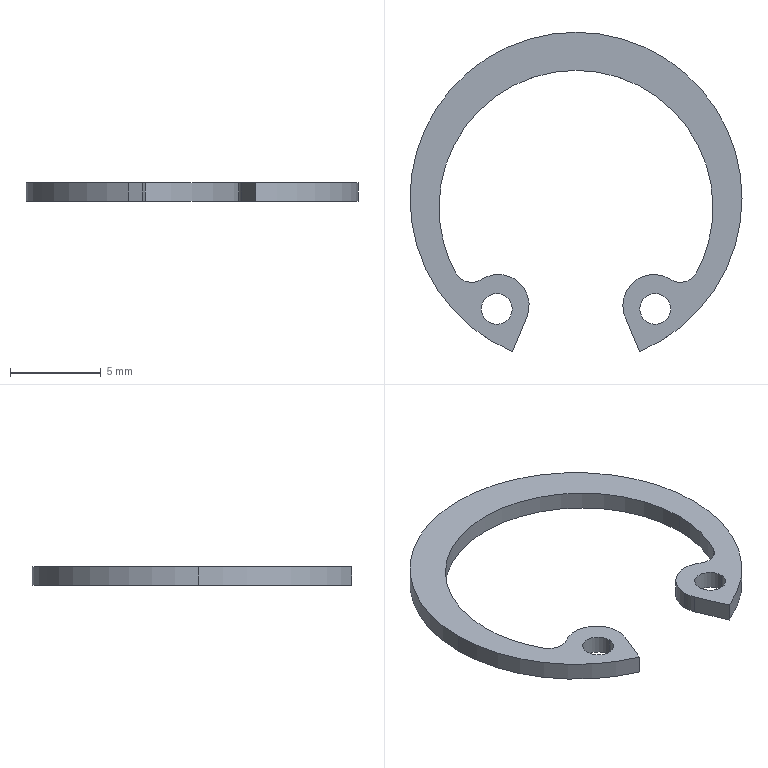Part | NX | features BREP 1 | 1 solid | 19 faces | box 18.3 x 17.603 x 1 mm | volume 85.781 mm3 | cylinder 15 | plane 4 | commonest cylinder face diameters 1.7 x4 3.4 x3 15.1 x3 18.3 x3 2 x2
STEP:
#1=CARTESIAN_POINT('',(-2.713,-6.549,-0.5));
#2=VERTEX_POINT('',#1);
#3=CARTESIAN_POINT('',(-5.208,-4.472,-0.5));
#4=VERTEX_POINT('',#3);
#5=CARTESIAN_POINT('',(-4.283,-5.899,-0.5));
#6=DIRECTION('',(0.,0.,1.));
#7=DIRECTION('',(1.,0.,0.));
#8=AXIS2_PLACEMENT_3D('',#5,#6,#7);
#9=CIRCLE('',#8,1.7);
#10=EDGE_CURVE('',#2,#4,#9,.T.);
#11=ORIENTED_EDGE('',*,*,#10,.F.);
#12=CARTESIAN_POINT('',(-3.502,-8.453,-0.5));
#13=VERTEX_POINT('',#12);
#14=CARTESIAN_POINT('',(-2.713,-6.549,-0.5));
#15=DIRECTION('',(0.3827,0.9239,0.));
#16=VECTOR('',#15,1000.);
#17=LINE('',#14,#16);
#18=EDGE_CURVE('',#13,#2,#17,.T.);
#19=ORIENTED_EDGE('',*,*,#18,.F.);
#20=CARTESIAN_POINT('',(-9.15,0.,-0.5));
#21=VERTEX_POINT('',#20);
#22=CARTESIAN_POINT('',(0.,0.,-0.5));
#23=DIRECTION('',(0.,0.,1.));
#24=DIRECTION('',(1.,0.,0.));
#25=AXIS2_PLACEMENT_3D('',#22,#23,#24);
#26=CIRCLE('',#25,9.15);
#27=EDGE_CURVE('',#21,#13,#26,.T.);
#28=ORIENTED_EDGE('',*,*,#27,.F.);
#29=CARTESIAN_POINT('',(9.15,0.,-0.5));
#30=VERTEX_POINT('',#29);
#31=CARTESIAN_POINT('',(0.,0.,-0.5));
#32=DIRECTION('',(0.,0.,1.));
#33=DIRECTION('',(1.,0.,0.));
#34=AXIS2_PLACEMENT_3D('',#31,#32,#33);
#35=CIRCLE('',#34,9.15);
#36=EDGE_CURVE('',#30,#21,#35,.T.);
#37=ORIENTED_EDGE('',*,*,#36,.F.);
#38=CARTESIAN_POINT('',(3.502,-8.453,-0.5));
#39=VERTEX_POINT('',#38);
#40=CARTESIAN_POINT('',(0.,0.,-0.5));
#41=DIRECTION('',(0.,0.,1.));
#42=DIRECTION('',(1.,0.,0.));
#43=AXIS2_PLACEMENT_3D('',#40,#41,#42);
#44=CIRCLE('',#43,9.15);
#45=EDGE_CURVE('',#39,#30,#44,.T.);
#46=ORIENTED_EDGE('',*,*,#45,.F.);
#47=CARTESIAN_POINT('',(2.713,-6.549,-0.5));
#48=VERTEX_POINT('',#47);
#49=CARTESIAN_POINT('',(2.713,-6.549,-0.5));
#50=DIRECTION('',(0.3827,-0.9239,0.));
#51=VECTOR('',#50,1000.);
#52=LINE('',#49,#51);
#53=EDGE_CURVE('',#48,#39,#52,.T.);
#54=ORIENTED_EDGE('',*,*,#53,.F.);
#55=CARTESIAN_POINT('',(2.583,-5.899,-0.5));
#56=VERTEX_POINT('',#55);
#57=CARTESIAN_POINT('',(4.283,-5.899,-0.5));
#58=DIRECTION('',(0.,0.,1.));
#59=DIRECTION('',(-1.,0.,0.));
#60=AXIS2_PLACEMENT_3D('',#57,#58,#59);
#61=CIRCLE('',#60,1.7);
#62=EDGE_CURVE('',#56,#48,#61,.T.);
#63=ORIENTED_EDGE('',*,*,#62,.F.);
#64=CARTESIAN_POINT('',(5.208,-4.472,-0.5));
#65=VERTEX_POINT('',#64);
#66=CARTESIAN_POINT('',(4.283,-5.899,-0.5));
#67=DIRECTION('',(0.,0.,1.));
#68=DIRECTION('',(-1.,0.,0.));
#69=AXIS2_PLACEMENT_3D('',#66,#67,#68);
#70=CIRCLE('',#69,1.7);
#71=EDGE_CURVE('',#65,#56,#70,.T.);
#72=ORIENTED_EDGE('',*,*,#71,.F.);
#73=CARTESIAN_POINT('',(6.63,-4.112,-0.5));
#74=VERTEX_POINT('',#73);
#75=CARTESIAN_POINT('',(5.752,-3.633,-0.5));
#76=DIRECTION('',(0.,0.,-1.));
#77=DIRECTION('',(1.,0.,0.));
#78=AXIS2_PLACEMENT_3D('',#75,#76,#77);
#79=CIRCLE('',#78,1.);
#80=EDGE_CURVE('',#74,#65,#79,.T.);
#81=ORIENTED_EDGE('',*,*,#80,.F.);
#82=CARTESIAN_POINT('',(7.55,-0.5,-0.5));
#83=VERTEX_POINT('',#82);
#84=CARTESIAN_POINT('',(0.,-0.5,-0.5));
#85=DIRECTION('',(0.,0.,-1.));
#86=DIRECTION('',(1.,0.,0.));
#87=AXIS2_PLACEMENT_3D('',#84,#85,#86);
#88=CIRCLE('',#87,7.55);
#89=EDGE_CURVE('',#83,#74,#88,.T.);
#90=ORIENTED_EDGE('',*,*,#89,.F.);
#91=CARTESIAN_POINT('',(-7.55,-0.5,-0.5));
#92=VERTEX_POINT('',#91);
#93=CARTESIAN_POINT('',(0.,-0.5,-0.5));
#94=DIRECTION('',(0.,0.,-1.));
#95=DIRECTION('',(1.,0.,0.));
#96=AXIS2_PLACEMENT_3D('',#93,#94,#95);
#97=CIRCLE('',#96,7.55);
#98=EDGE_CURVE('',#92,#83,#97,.T.);
#99=ORIENTED_EDGE('',*,*,#98,.F.);
#100=CARTESIAN_POINT('',(-6.63,-4.112,-0.5));
#101=VERTEX_POINT('',#100);
#102=CARTESIAN_POINT('',(0.,-0.5,-0.5));
#103=DIRECTION('',(0.,0.,-1.));
#104=DIRECTION('',(1.,0.,0.));
#105=AXIS2_PLACEMENT_3D('',#102,#103,#104);
#106=CIRCLE('',#105,7.55);
#107=EDGE_CURVE('',#101,#92,#106,.T.);
#108=ORIENTED_EDGE('',*,*,#107,.F.);
#109=CARTESIAN_POINT('',(-5.752,-3.633,-0.5));
#110=DIRECTION('',(0.,0.,-1.));
#111=DIRECTION('',(-1.,0.,0.));
#112=AXIS2_PLACEMENT_3D('',#109,#110,#111);
#113=CIRCLE('',#112,1.);
#114=EDGE_CURVE('',#4,#101,#113,.T.);
#115=ORIENTED_EDGE('',*,*,#114,.F.);
#116=EDGE_LOOP('',(#11,#19,#28,#37,#46,#54,#63,#72,#81,#90,#99,#108,#115));
#117=FACE_BOUND('',#116,.T.);
#118=CARTESIAN_POINT('',(-5.216,-6.098,-0.5));
#119=VERTEX_POINT('',#118);
#120=CARTESIAN_POINT('',(-3.516,-6.098,-0.5));
#121=VERTEX_POINT('',#120);
#122=CARTESIAN_POINT('',(-4.366,-6.098,-0.5));
#123=DIRECTION('',(0.,0.,1.));
#124=DIRECTION('',(1.,0.,0.));
#125=AXIS2_PLACEMENT_3D('',#122,#123,#124);
#126=CIRCLE('',#125,0.85);
#127=EDGE_CURVE('',#119,#121,#126,.T.);
#128=ORIENTED_EDGE('',*,*,#127,.T.);
#129=CARTESIAN_POINT('',(-4.366,-6.098,-0.5));
#130=DIRECTION('',(0.,0.,1.));
#131=DIRECTION('',(1.,0.,0.));
#132=AXIS2_PLACEMENT_3D('',#129,#130,#131);
#133=CIRCLE('',#132,0.85);
#134=EDGE_CURVE('',#121,#119,#133,.T.);
#135=ORIENTED_EDGE('',*,*,#134,.T.);
#136=EDGE_LOOP('',(#128,#135));
#137=FACE_BOUND('',#136,.T.);
#138=CARTESIAN_POINT('',(3.516,-6.098,-0.5));
#139=VERTEX_POINT('',#138);
#140=CARTESIAN_POINT('',(5.216,-6.098,-0.5));
#141=VERTEX_POINT('',#140);
#142=CARTESIAN_POINT('',(4.366,-6.098,-0.5));
#143=DIRECTION('',(0.,0.,1.));
#144=DIRECTION('',(-1.,0.,0.));
#145=AXIS2_PLACEMENT_3D('',#142,#143,#144);
#146=CIRCLE('',#145,0.85);
#147=EDGE_CURVE('',#139,#141,#146,.T.);
#148=ORIENTED_EDGE('',*,*,#147,.T.);
#149=CARTESIAN_POINT('',(4.366,-6.098,-0.5));
#150=DIRECTION('',(0.,0.,1.));
#151=DIRECTION('',(-1.,0.,0.));
#152=AXIS2_PLACEMENT_3D('',#149,#150,#151);
#153=CIRCLE('',#152,0.85);
#154=EDGE_CURVE('',#141,#139,#153,.T.);
#155=ORIENTED_EDGE('',*,*,#154,.T.);
#156=EDGE_LOOP('',(#148,#155));
#157=FACE_BOUND('',#156,.T.);
#158=CARTESIAN_POINT('',(-4.283,-5.899,-0.5));
#159=DIRECTION('',(0.,0.,1.));
#160=DIRECTION('',(1.,0.,0.));
#161=AXIS2_PLACEMENT_3D('',#158,#159,#160);
#162=PLANE('',#161);
#163=ADVANCED_FACE('',(#117,#137,#157),#162,.F.);
#164=CARTESIAN_POINT('',(5.216,-6.098,0.5));
#165=VERTEX_POINT('',#164);
#166=CARTESIAN_POINT('',(5.216,-6.098,0.5));
#167=DIRECTION('',(0.,0.,-1.));
#168=VECTOR('',#167,1000.);
#169=LINE('',#166,#168);
#170=EDGE_CURVE('',#165,#141,#169,.T.);
#171=ORIENTED_EDGE('',*,*,#170,.F.);
#172=CARTESIAN_POINT('',(3.516,-6.098,0.5));
#173=VERTEX_POINT('',#172);
#174=CARTESIAN_POINT('',(4.366,-6.098,0.5));
#175=DIRECTION('',(0.,0.,1.));
#176=DIRECTION('',(-1.,0.,0.));
#177=AXIS2_PLACEMENT_3D('',#174,#175,#176);
#178=CIRCLE('',#177,0.85);
#179=EDGE_CURVE('',#165,#173,#178,.T.);
#180=ORIENTED_EDGE('',*,*,#179,.T.);
#181=CARTESIAN_POINT('',(3.516,-6.098,0.5));
#182=DIRECTION('',(0.,0.,-1.));
#183=VECTOR('',#182,1000.);
#184=LINE('',#181,#183);
#185=EDGE_CURVE('',#173,#139,#184,.T.);
#186=ORIENTED_EDGE('',*,*,#185,.T.);
#187=ORIENTED_EDGE('',*,*,#154,.F.);
#188=EDGE_LOOP('',(#171,#180,#186,#187));
#189=FACE_BOUND('',#188,.T.);
#190=CARTESIAN_POINT('',(4.366,-6.098,0.5));
#191=DIRECTION('',(0.,0.,-1.));
#192=DIRECTION('',(-1.,0.,0.));
#193=AXIS2_PLACEMENT_3D('',#190,#191,#192);
#194=CYLINDRICAL_SURFACE('',#193,0.85);
#195=ADVANCED_FACE('',(#189),#194,.F.);
#196=CARTESIAN_POINT('',(-3.516,-6.098,0.5));
#197=VERTEX_POINT('',#196);
#198=CARTESIAN_POINT('',(-3.516,-6.098,0.5));
#199=DIRECTION('',(0.,0.,-1.));
#200=VECTOR('',#199,1000.);
#201=LINE('',#198,#200);
#202=EDGE_CURVE('',#197,#121,#201,.T.);
#203=ORIENTED_EDGE('',*,*,#202,.F.);
#204=CARTESIAN_POINT('',(-5.216,-6.098,0.5));
#205=VERTEX_POINT('',#204);
#206=CARTESIAN_POINT('',(-4.366,-6.098,0.5));
#207=DIRECTION('',(0.,0.,1.));
#208=DIRECTION('',(1.,0.,0.));
#209=AXIS2_PLACEMENT_3D('',#206,#207,#208);
#210=CIRCLE('',#209,0.85);
#211=EDGE_CURVE('',#197,#205,#210,.T.);
#212=ORIENTED_EDGE('',*,*,#211,.T.);
#213=CARTESIAN_POINT('',(-5.216,-6.098,0.5));
#214=DIRECTION('',(0.,0.,-1.));
#215=VECTOR('',#214,1000.);
#216=LINE('',#213,#215);
#217=EDGE_CURVE('',#205,#119,#216,.T.);
#218=ORIENTED_EDGE('',*,*,#217,.T.);
#219=ORIENTED_EDGE('',*,*,#134,.F.);
#220=EDGE_LOOP('',(#203,#212,#218,#219));
#221=FACE_BOUND('',#220,.T.);
#222=CARTESIAN_POINT('',(-4.366,-6.098,0.5));
#223=DIRECTION('',(0.,0.,-1.));
#224=DIRECTION('',(-1.,0.,0.));
#225=AXIS2_PLACEMENT_3D('',#222,#223,#224);
#226=CYLINDRICAL_SURFACE('',#225,0.85);
#227=ADVANCED_FACE('',(#221),#226,.F.);
#228=CARTESIAN_POINT('',(-3.502,-8.453,0.5));
#229=VERTEX_POINT('',#228);
#230=CARTESIAN_POINT('',(-3.502,-8.453,0.5));
#231=DIRECTION('',(0.,0.,-1.));
#232=VECTOR('',#231,1000.);
#233=LINE('',#230,#232);
#234=EDGE_CURVE('',#229,#13,#233,.T.);
#235=ORIENTED_EDGE('',*,*,#234,.T.);
#236=ORIENTED_EDGE('',*,*,#18,.T.);
#237=CARTESIAN_POINT('',(-2.713,-6.549,0.5));
#238=VERTEX_POINT('',#237);
#239=CARTESIAN_POINT('',(-2.713,-6.549,0.5));
#240=DIRECTION('',(0.,0.,-1.));
#241=VECTOR('',#240,1000.);
#242=LINE('',#239,#241);
#243=EDGE_CURVE('',#238,#2,#242,.T.);
#244=ORIENTED_EDGE('',*,*,#243,.F.);
#245=CARTESIAN_POINT('',(-2.713,-6.549,0.5));
#246=DIRECTION('',(0.3827,0.9239,0.));
#247=VECTOR('',#246,1000.);
#248=LINE('',#245,#247);
#249=EDGE_CURVE('',#229,#238,#248,.T.);
#250=ORIENTED_EDGE('',*,*,#249,.F.);
#251=EDGE_LOOP('',(#235,#236,#244,#250));
#252=FACE_BOUND('',#251,.T.);
#253=CARTESIAN_POINT('',(-2.713,-6.549,0.5));
#254=DIRECTION('',(-0.9239,0.3827,0.));
#255=DIRECTION('',(-0.3827,-0.9239,0.));
#256=AXIS2_PLACEMENT_3D('',#253,#254,#255);
#257=PLANE('',#256);
#258=ADVANCED_FACE('',(#252),#257,.F.);
#259=CARTESIAN_POINT('',(9.15,0.,0.5));
#260=VERTEX_POINT('',#259);
#261=CARTESIAN_POINT('',(9.15,0.,0.5));
#262=DIRECTION('',(0.,0.,-1.));
#263=VECTOR('',#262,1000.);
#264=LINE('',#261,#263);
#265=EDGE_CURVE('',#260,#30,#264,.T.);
#266=ORIENTED_EDGE('',*,*,#265,.F.);
#267=CARTESIAN_POINT('',(3.502,-8.453,0.5));
#268=VERTEX_POINT('',#267);
#269=CARTESIAN_POINT('',(0.,0.,0.5));
#270=DIRECTION('',(0.,0.,1.));
#271=DIRECTION('',(1.,0.,0.));
#272=AXIS2_PLACEMENT_3D('',#269,#270,#271);
#273=CIRCLE('',#272,9.15);
#274=EDGE_CURVE('',#268,#260,#273,.T.);
#275=ORIENTED_EDGE('',*,*,#274,.F.);
#276=CARTESIAN_POINT('',(3.502,-8.453,0.5));
#277=DIRECTION('',(0.,0.,-1.));
#278=VECTOR('',#277,1000.);
#279=LINE('',#276,#278);
#280=EDGE_CURVE('',#268,#39,#279,.T.);
#281=ORIENTED_EDGE('',*,*,#280,.T.);
#282=ORIENTED_EDGE('',*,*,#45,.T.);
#283=EDGE_LOOP('',(#266,#275,#281,#282));
#284=FACE_BOUND('',#283,.T.);
#285=CARTESIAN_POINT('',(0.,0.,0.5));
#286=DIRECTION('',(0.,0.,-1.));
#287=DIRECTION('',(-1.,0.,0.));
#288=AXIS2_PLACEMENT_3D('',#285,#286,#287);
#289=CYLINDRICAL_SURFACE('',#288,9.15);
#290=ADVANCED_FACE('',(#284),#289,.T.);
#291=CARTESIAN_POINT('',(2.713,-6.549,0.5));
#292=VERTEX_POINT('',#291);
#293=CARTESIAN_POINT('',(2.713,-6.549,0.5));
#294=DIRECTION('',(0.,0.,-1.));
#295=VECTOR('',#294,1000.);
#296=LINE('',#293,#295);
#297=EDGE_CURVE('',#292,#48,#296,.T.);
#298=ORIENTED_EDGE('',*,*,#297,.T.);
#299=ORIENTED_EDGE('',*,*,#53,.T.);
#300=ORIENTED_EDGE('',*,*,#280,.F.);
#301=CARTESIAN_POINT('',(2.713,-6.549,0.5));
#302=DIRECTION('',(0.3827,-0.9239,0.));
#303=VECTOR('',#302,1000.);
#304=LINE('',#301,#303);
#305=EDGE_CURVE('',#292,#268,#304,.T.);
#306=ORIENTED_EDGE('',*,*,#305,.F.);
#307=EDGE_LOOP('',(#298,#299,#300,#306));
#308=FACE_BOUND('',#307,.T.);
#309=CARTESIAN_POINT('',(2.713,-6.549,0.5));
#310=DIRECTION('',(0.9239,0.3827,0.));
#311=DIRECTION('',(-0.3827,0.9239,0.));
#312=AXIS2_PLACEMENT_3D('',#309,#310,#311);
#313=PLANE('',#312);
#314=ADVANCED_FACE('',(#308),#313,.F.);
#315=CARTESIAN_POINT('',(2.583,-5.899,0.5));
#316=VERTEX_POINT('',#315);
#317=CARTESIAN_POINT('',(2.583,-5.899,0.5));
#318=DIRECTION('',(0.,0.,-1.));
#319=VECTOR('',#318,1000.);
#320=LINE('',#317,#319);
#321=EDGE_CURVE('',#316,#56,#320,.T.);
#322=ORIENTED_EDGE('',*,*,#321,.F.);
#323=CARTESIAN_POINT('',(5.208,-4.472,0.5));
#324=VERTEX_POINT('',#323);
#325=CARTESIAN_POINT('',(4.283,-5.899,0.5));
#326=DIRECTION('',(0.,0.,1.));
#327=DIRECTION('',(-1.,0.,0.));
#328=AXIS2_PLACEMENT_3D('',#325,#326,#327);
#329=CIRCLE('',#328,1.7);
#330=EDGE_CURVE('',#324,#316,#329,.T.);
#331=ORIENTED_EDGE('',*,*,#330,.F.);
#332=CARTESIAN_POINT('',(5.208,-4.472,0.5));
#333=DIRECTION('',(0.,0.,-1.));
#334=VECTOR('',#333,1000.);
#335=LINE('',#332,#334);
#336=EDGE_CURVE('',#324,#65,#335,.T.);
#337=ORIENTED_EDGE('',*,*,#336,.T.);
#338=ORIENTED_EDGE('',*,*,#71,.T.);
#339=EDGE_LOOP('',(#322,#331,#337,#338));
#340=FACE_BOUND('',#339,.T.);
#341=CARTESIAN_POINT('',(4.283,-5.899,0.5));
#342=DIRECTION('',(0.,0.,-1.));
#343=DIRECTION('',(-1.,0.,0.));
#344=AXIS2_PLACEMENT_3D('',#341,#342,#343);
#345=CYLINDRICAL_SURFACE('',#344,1.7);
#346=ADVANCED_FACE('',(#340),#345,.T.);
#347=CARTESIAN_POINT('',(6.63,-4.112,0.5));
#348=VERTEX_POINT('',#347);
#349=CARTESIAN_POINT('',(6.63,-4.112,0.5));
#350=DIRECTION('',(0.,0.,-1.));
#351=VECTOR('',#350,1000.);
#352=LINE('',#349,#351);
#353=EDGE_CURVE('',#348,#74,#352,.T.);
#354=ORIENTED_EDGE('',*,*,#353,.T.);
#355=ORIENTED_EDGE('',*,*,#80,.T.);
#356=ORIENTED_EDGE('',*,*,#336,.F.);
#357=CARTESIAN_POINT('',(5.752,-3.633,0.5));
#358=DIRECTION('',(0.,0.,-1.));
#359=DIRECTION('',(1.,0.,0.));
#360=AXIS2_PLACEMENT_3D('',#357,#358,#359);
#361=CIRCLE('',#360,1.);
#362=EDGE_CURVE('',#348,#324,#361,.T.);
#363=ORIENTED_EDGE('',*,*,#362,.F.);
#364=EDGE_LOOP('',(#354,#355,#356,#363));
#365=FACE_BOUND('',#364,.T.);
#366=CARTESIAN_POINT('',(5.752,-3.633,0.5));
#367=DIRECTION('',(0.,0.,-1.));
#368=DIRECTION('',(-1.,0.,0.));
#369=AXIS2_PLACEMENT_3D('',#366,#367,#368);
#370=CYLINDRICAL_SURFACE('',#369,1.);
#371=ADVANCED_FACE('',(#365),#370,.F.);
#372=CARTESIAN_POINT('',(-7.55,-0.5,0.5));
#373=VERTEX_POINT('',#372);
#374=CARTESIAN_POINT('',(-7.55,-0.5,0.5));
#375=DIRECTION('',(0.,0.,-1.));
#376=VECTOR('',#375,1000.);
#377=LINE('',#374,#376);
#378=EDGE_CURVE('',#373,#92,#377,.T.);
#379=ORIENTED_EDGE('',*,*,#378,.F.);
#380=CARTESIAN_POINT('',(-6.63,-4.112,0.5));
#381=VERTEX_POINT('',#380);
#382=CARTESIAN_POINT('',(0.,-0.5,0.5));
#383=DIRECTION('',(0.,0.,-1.));
#384=DIRECTION('',(1.,0.,0.));
#385=AXIS2_PLACEMENT_3D('',#382,#383,#384);
#386=CIRCLE('',#385,7.55);
#387=EDGE_CURVE('',#381,#373,#386,.T.);
#388=ORIENTED_EDGE('',*,*,#387,.F.);
#389=CARTESIAN_POINT('',(-6.63,-4.112,0.5));
#390=DIRECTION('',(0.,0.,-1.));
#391=VECTOR('',#390,1000.);
#392=LINE('',#389,#391);
#393=EDGE_CURVE('',#381,#101,#392,.T.);
#394=ORIENTED_EDGE('',*,*,#393,.T.);
#395=ORIENTED_EDGE('',*,*,#107,.T.);
#396=EDGE_LOOP('',(#379,#388,#394,#395));
#397=FACE_BOUND('',#396,.T.);
#398=CARTESIAN_POINT('',(0.,-0.5,0.5));
#399=DIRECTION('',(0.,0.,-1.));
#400=DIRECTION('',(-1.,0.,0.));
#401=AXIS2_PLACEMENT_3D('',#398,#399,#400);
#402=CYLINDRICAL_SURFACE('',#401,7.55);
#403=ADVANCED_FACE('',(#397),#402,.F.);
#404=CARTESIAN_POINT('',(-5.208,-4.472,0.5));
#405=VERTEX_POINT('',#404);
#406=CARTESIAN_POINT('',(-5.208,-4.472,0.5));
#407=DIRECTION('',(0.,0.,-1.));
#408=VECTOR('',#407,1000.);
#409=LINE('',#406,#408);
#410=EDGE_CURVE('',#405,#4,#409,.T.);
#411=ORIENTED_EDGE('',*,*,#410,.T.);
#412=ORIENTED_EDGE('',*,*,#114,.T.);
#413=ORIENTED_EDGE('',*,*,#393,.F.);
#414=CARTESIAN_POINT('',(-5.752,-3.633,0.5));
#415=DIRECTION('',(0.,0.,-1.));
#416=DIRECTION('',(-1.,0.,0.));
#417=AXIS2_PLACEMENT_3D('',#414,#415,#416);
#418=CIRCLE('',#417,1.);
#419=EDGE_CURVE('',#405,#381,#418,.T.);
#420=ORIENTED_EDGE('',*,*,#419,.F.);
#421=EDGE_LOOP('',(#411,#412,#413,#420));
#422=FACE_BOUND('',#421,.T.);
#423=CARTESIAN_POINT('',(-5.752,-3.633,0.5));
#424=DIRECTION('',(0.,0.,-1.));
#425=DIRECTION('',(-1.,0.,0.));
#426=AXIS2_PLACEMENT_3D('',#423,#424,#425);
#427=CYLINDRICAL_SURFACE('',#426,1.);
#428=ADVANCED_FACE('',(#422),#427,.F.);
#429=ORIENTED_EDGE('',*,*,#243,.T.);
#430=ORIENTED_EDGE('',*,*,#10,.T.);
#431=ORIENTED_EDGE('',*,*,#410,.F.);
#432=CARTESIAN_POINT('',(-4.283,-5.899,0.5));
#433=DIRECTION('',(0.,0.,1.));
#434=DIRECTION('',(1.,0.,0.));
#435=AXIS2_PLACEMENT_3D('',#432,#433,#434);
#436=CIRCLE('',#435,1.7);
#437=EDGE_CURVE('',#238,#405,#436,.T.);
#438=ORIENTED_EDGE('',*,*,#437,.F.);
#439=EDGE_LOOP('',(#429,#430,#431,#438));
#440=FACE_BOUND('',#439,.T.);
#441=CARTESIAN_POINT('',(-4.283,-5.899,0.5));
#442=DIRECTION('',(0.,0.,-1.));
#443=DIRECTION('',(-1.,0.,0.));
#444=AXIS2_PLACEMENT_3D('',#441,#442,#443);
#445=CYLINDRICAL_SURFACE('',#444,1.7);
#446=ADVANCED_FACE('',(#440),#445,.T.);
#447=CARTESIAN_POINT('',(4.366,-6.098,0.5));
#448=DIRECTION('',(0.,0.,1.));
#449=DIRECTION('',(-1.,0.,0.));
#450=AXIS2_PLACEMENT_3D('',#447,#448,#449);
#451=CIRCLE('',#450,0.85);
#452=EDGE_CURVE('',#173,#165,#451,.T.);
#453=ORIENTED_EDGE('',*,*,#452,.F.);
#454=ORIENTED_EDGE('',*,*,#179,.F.);
#455=EDGE_LOOP('',(#453,#454));
#456=FACE_BOUND('',#455,.T.);
#457=ORIENTED_EDGE('',*,*,#437,.T.);
#458=ORIENTED_EDGE('',*,*,#419,.T.);
#459=ORIENTED_EDGE('',*,*,#387,.T.);
#460=CARTESIAN_POINT('',(7.55,-0.5,0.5));
#461=VERTEX_POINT('',#460);
#462=CARTESIAN_POINT('',(0.,-0.5,0.5));
#463=DIRECTION('',(0.,0.,-1.));
#464=DIRECTION('',(1.,0.,0.));
#465=AXIS2_PLACEMENT_3D('',#462,#463,#464);
#466=CIRCLE('',#465,7.55);
#467=EDGE_CURVE('',#373,#461,#466,.T.);
#468=ORIENTED_EDGE('',*,*,#467,.T.);
#469=CARTESIAN_POINT('',(0.,-0.5,0.5));
#470=DIRECTION('',(0.,0.,-1.));
#471=DIRECTION('',(1.,0.,0.));
#472=AXIS2_PLACEMENT_3D('',#469,#470,#471);
#473=CIRCLE('',#472,7.55);
#474=EDGE_CURVE('',#461,#348,#473,.T.);
#475=ORIENTED_EDGE('',*,*,#474,.T.);
#476=ORIENTED_EDGE('',*,*,#362,.T.);
#477=ORIENTED_EDGE('',*,*,#330,.T.);
#478=CARTESIAN_POINT('',(4.283,-5.899,0.5));
#479=DIRECTION('',(0.,0.,1.));
#480=DIRECTION('',(-1.,0.,0.));
#481=AXIS2_PLACEMENT_3D('',#478,#479,#480);
#482=CIRCLE('',#481,1.7);
#483=EDGE_CURVE('',#316,#292,#482,.T.);
#484=ORIENTED_EDGE('',*,*,#483,.T.);
#485=ORIENTED_EDGE('',*,*,#305,.T.);
#486=ORIENTED_EDGE('',*,*,#274,.T.);
#487=CARTESIAN_POINT('',(-9.15,0.,0.5));
#488=VERTEX_POINT('',#487);
#489=CARTESIAN_POINT('',(0.,0.,0.5));
#490=DIRECTION('',(0.,0.,1.));
#491=DIRECTION('',(1.,0.,0.));
#492=AXIS2_PLACEMENT_3D('',#489,#490,#491);
#493=CIRCLE('',#492,9.15);
#494=EDGE_CURVE('',#260,#488,#493,.T.);
#495=ORIENTED_EDGE('',*,*,#494,.T.);
#496=CARTESIAN_POINT('',(0.,0.,0.5));
#497=DIRECTION('',(0.,0.,1.));
#498=DIRECTION('',(1.,0.,0.));
#499=AXIS2_PLACEMENT_3D('',#496,#497,#498);
#500=CIRCLE('',#499,9.15);
#501=EDGE_CURVE('',#488,#229,#500,.T.);
#502=ORIENTED_EDGE('',*,*,#501,.T.);
#503=ORIENTED_EDGE('',*,*,#249,.T.);
#504=EDGE_LOOP('',(#457,#458,#459,#468,#475,#476,#477,#484,#485,#486,#495,#502,#503));
#505=FACE_BOUND('',#504,.T.);
#506=CARTESIAN_POINT('',(-4.366,-6.098,0.5));
#507=DIRECTION('',(0.,0.,1.));
#508=DIRECTION('',(1.,0.,0.));
#509=AXIS2_PLACEMENT_3D('',#506,#507,#508);
#510=CIRCLE('',#509,0.85);
#511=EDGE_CURVE('',#205,#197,#510,.T.);
#512=ORIENTED_EDGE('',*,*,#511,.F.);
#513=ORIENTED_EDGE('',*,*,#211,.F.);
#514=EDGE_LOOP('',(#512,#513));
#515=FACE_BOUND('',#514,.T.);
#516=CARTESIAN_POINT('',(-4.283,-5.899,0.5));
#517=DIRECTION('',(0.,0.,1.));
#518=DIRECTION('',(1.,0.,0.));
#519=AXIS2_PLACEMENT_3D('',#516,#517,#518);
#520=PLANE('',#519);
#521=ADVANCED_FACE('',(#456,#505,#515),#520,.T.);
#522=CARTESIAN_POINT('',(7.55,-0.5,0.5));
#523=DIRECTION('',(0.,0.,-1.));
#524=VECTOR('',#523,1000.);
#525=LINE('',#522,#524);
#526=EDGE_CURVE('',#461,#83,#525,.T.);
#527=ORIENTED_EDGE('',*,*,#526,.F.);
#528=ORIENTED_EDGE('',*,*,#467,.F.);
#529=ORIENTED_EDGE('',*,*,#378,.T.);
#530=ORIENTED_EDGE('',*,*,#98,.T.);
#531=EDGE_LOOP('',(#527,#528,#529,#530));
#532=FACE_BOUND('',#531,.T.);
#533=CARTESIAN_POINT('',(0.,-0.5,0.5));
#534=DIRECTION('',(0.,0.,-1.));
#535=DIRECTION('',(-1.,0.,0.));
#536=AXIS2_PLACEMENT_3D('',#533,#534,#535);
#537=CYLINDRICAL_SURFACE('',#536,7.55);
#538=ADVANCED_FACE('',(#532),#537,.F.);
#539=ORIENTED_EDGE('',*,*,#474,.F.);
#540=ORIENTED_EDGE('',*,*,#526,.T.);
#541=ORIENTED_EDGE('',*,*,#89,.T.);
#542=ORIENTED_EDGE('',*,*,#353,.F.);
#543=EDGE_LOOP('',(#539,#540,#541,#542));
#544=FACE_BOUND('',#543,.T.);
#545=CARTESIAN_POINT('',(0.,-0.5,0.5));
#546=DIRECTION('',(0.,0.,-1.));
#547=DIRECTION('',(-1.,0.,0.));
#548=AXIS2_PLACEMENT_3D('',#545,#546,#547);
#549=CYLINDRICAL_SURFACE('',#548,7.55);
#550=ADVANCED_FACE('',(#544),#549,.F.);
#551=ORIENTED_EDGE('',*,*,#483,.F.);
#552=ORIENTED_EDGE('',*,*,#321,.T.);
#553=ORIENTED_EDGE('',*,*,#62,.T.);
#554=ORIENTED_EDGE('',*,*,#297,.F.);
#555=EDGE_LOOP('',(#551,#552,#553,#554));
#556=FACE_BOUND('',#555,.T.);
#557=CARTESIAN_POINT('',(4.283,-5.899,0.5));
#558=DIRECTION('',(0.,0.,-1.));
#559=DIRECTION('',(-1.,0.,0.));
#560=AXIS2_PLACEMENT_3D('',#557,#558,#559);
#561=CYLINDRICAL_SURFACE('',#560,1.7);
#562=ADVANCED_FACE('',(#556),#561,.T.);
#563=ORIENTED_EDGE('',*,*,#501,.F.);
#564=CARTESIAN_POINT('',(-9.15,0.,0.5));
#565=DIRECTION('',(0.,0.,-1.));
#566=VECTOR('',#565,1000.);
#567=LINE('',#564,#566);
#568=EDGE_CURVE('',#488,#21,#567,.T.);
#569=ORIENTED_EDGE('',*,*,#568,.T.);
#570=ORIENTED_EDGE('',*,*,#27,.T.);
#571=ORIENTED_EDGE('',*,*,#234,.F.);
#572=EDGE_LOOP('',(#563,#569,#570,#571));
#573=FACE_BOUND('',#572,.T.);
#574=CARTESIAN_POINT('',(0.,0.,0.5));
#575=DIRECTION('',(0.,0.,-1.));
#576=DIRECTION('',(-1.,0.,0.));
#577=AXIS2_PLACEMENT_3D('',#574,#575,#576);
#578=CYLINDRICAL_SURFACE('',#577,9.15);
#579=ADVANCED_FACE('',(#573),#578,.T.);
#580=ORIENTED_EDGE('',*,*,#494,.F.);
#581=ORIENTED_EDGE('',*,*,#265,.T.);
#582=ORIENTED_EDGE('',*,*,#36,.T.);
#583=ORIENTED_EDGE('',*,*,#568,.F.);
#584=EDGE_LOOP('',(#580,#581,#582,#583));
#585=FACE_BOUND('',#584,.T.);
#586=CARTESIAN_POINT('',(0.,0.,0.5));
#587=DIRECTION('',(0.,0.,-1.));
#588=DIRECTION('',(-1.,0.,0.));
#589=AXIS2_PLACEMENT_3D('',#586,#587,#588);
#590=CYLINDRICAL_SURFACE('',#589,9.15);
#591=ADVANCED_FACE('',(#585),#590,.T.);
#592=ORIENTED_EDGE('',*,*,#511,.T.);
#593=ORIENTED_EDGE('',*,*,#202,.T.);
#594=ORIENTED_EDGE('',*,*,#127,.F.);
#595=ORIENTED_EDGE('',*,*,#217,.F.);
#596=EDGE_LOOP('',(#592,#593,#594,#595));
#597=FACE_BOUND('',#596,.T.);
#598=CARTESIAN_POINT('',(-4.366,-6.098,0.5));
#599=DIRECTION('',(0.,0.,-1.));
#600=DIRECTION('',(-1.,0.,0.));
#601=AXIS2_PLACEMENT_3D('',#598,#599,#600);
#602=CYLINDRICAL_SURFACE('',#601,0.85);
#603=ADVANCED_FACE('',(#597),#602,.F.);
#604=ORIENTED_EDGE('',*,*,#452,.T.);
#605=ORIENTED_EDGE('',*,*,#170,.T.);
#606=ORIENTED_EDGE('',*,*,#147,.F.);
#607=ORIENTED_EDGE('',*,*,#185,.F.);
#608=EDGE_LOOP('',(#604,#605,#606,#607));
#609=FACE_BOUND('',#608,.T.);
#610=CARTESIAN_POINT('',(4.366,-6.098,0.5));
#611=DIRECTION('',(0.,0.,-1.));
#612=DIRECTION('',(-1.,0.,0.));
#613=AXIS2_PLACEMENT_3D('',#610,#611,#612);
#614=CYLINDRICAL_SURFACE('',#613,0.85);
#615=ADVANCED_FACE('',(#609),#614,.F.);
#616=CLOSED_SHELL('',(#163,#195,#227,#258,#290,#314,#346,#371,#403,#428,#446,#521,#538,#550,#562,#579,#591,#603,#615));
#617=MANIFOLD_SOLID_BREP('',#616);
#618=(LENGTH_UNIT()NAMED_UNIT(*)SI_UNIT(.MILLI.,.METRE.));
#619=UNCERTAINTY_MEASURE_WITH_UNIT(LENGTH_MEASURE(0.00001),#618,'','');
#620=(NAMED_UNIT(*)PLANE_ANGLE_UNIT()SI_UNIT($,.RADIAN.));
#621=(NAMED_UNIT(*)SI_UNIT($,.STERADIAN.)SOLID_ANGLE_UNIT());
#622=(GEOMETRIC_REPRESENTATION_CONTEXT(3)GLOBAL_UNCERTAINTY_ASSIGNED_CONTEXT((#619))GLOBAL_UNIT_ASSIGNED_CONTEXT((#618,#620,#621))REPRESENTATION_CONTEXT('',''));
#623=ADVANCED_BREP_SHAPE_REPRESENTATION('',(#617),#622);